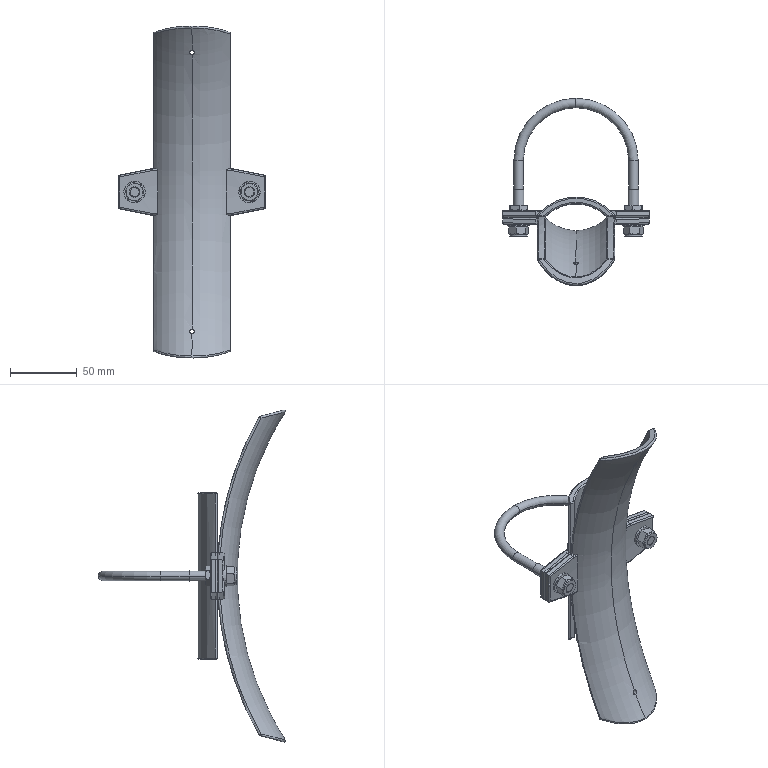Part | SolidWorks | 9 solids | 248 faces | box 110 x 140.16 x 248.72 mm | volume 144170 mm3 | cylinder 84 | plane 72 | cone 36 | torus 22 | sphere 22 | spline 12 | commonest cylinder face diameters 2 x34 6.647 x8 10 x8 3.3 x4 6.8 x4 7.1 x4